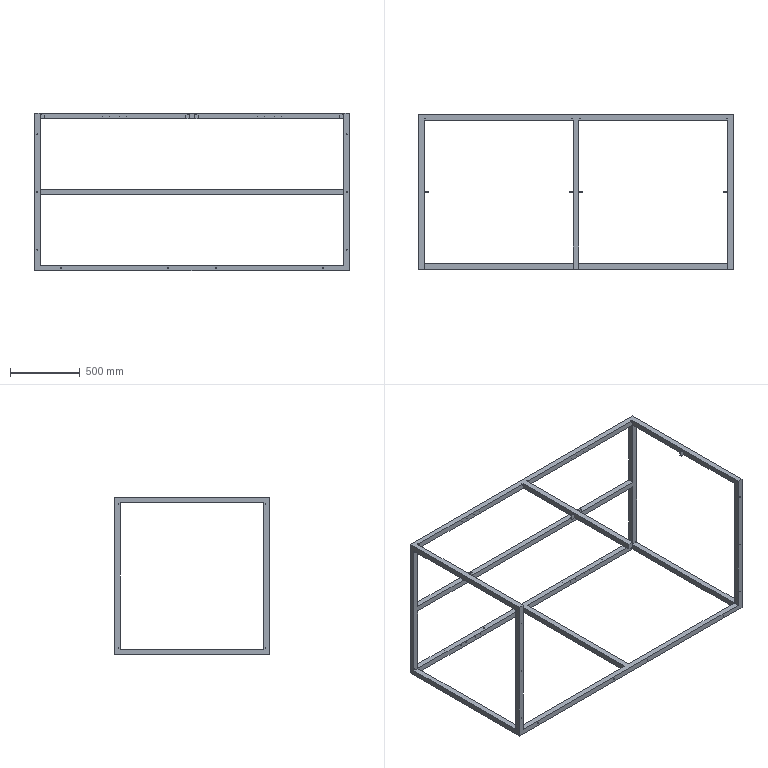Part | STEP file | 1 solid | 569 faces | box 2260 x 1110 x 1130 mm | volume 31144835 mm3 | cylinder 318 | cone 172 | plane 79 | commonest cylinder face diameters 2.5 x96 4.2 x64 7 x48 3.3 x36 10 x28 5 x24